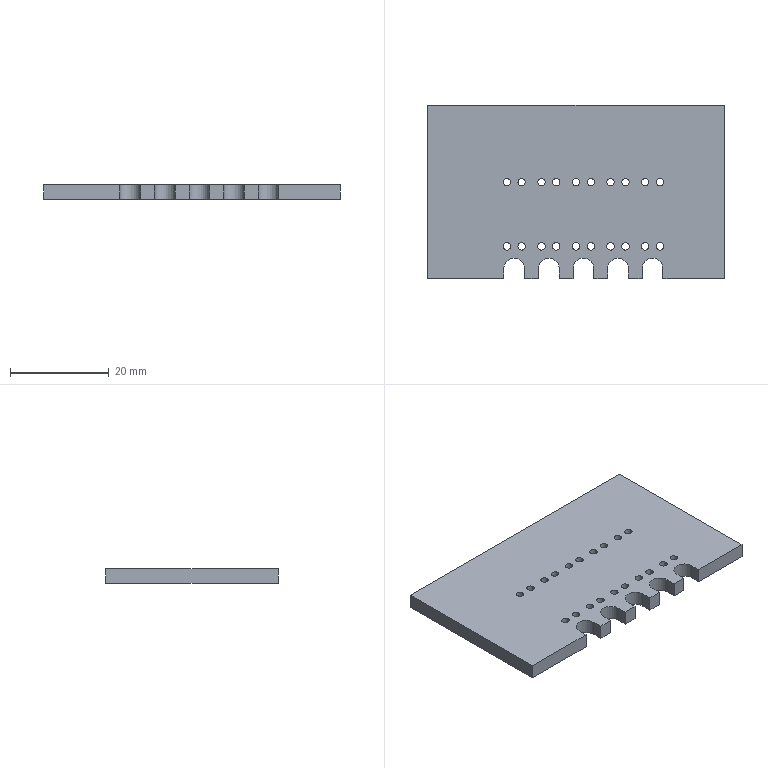Part | STEP file | 10000020453swp000-1 | 1 solid | 66 faces | box 60 x 35 x 3 mm | volume 5964 mm3 | cylinder 45 | plane 21 | commonest cylinder face diameters 1.5 x40 4.2 x5